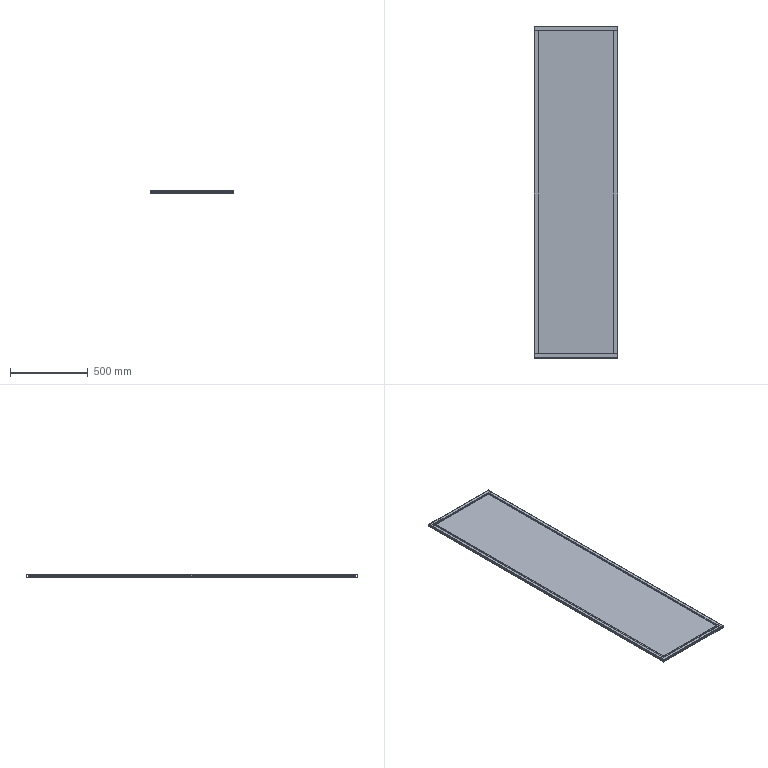Part | SolidWorks | features ICE 2, WeldMemberFeat 1, WeldmentFeature 1 | 5 solids | 167 faces | box 540 x 2136 x 18 mm | volume 11415432 mm3 | plane 98 | cylinder 69 | commonest cylinder face diameters 1.1 x24 3.6 x20 5.8 x20 1 x5